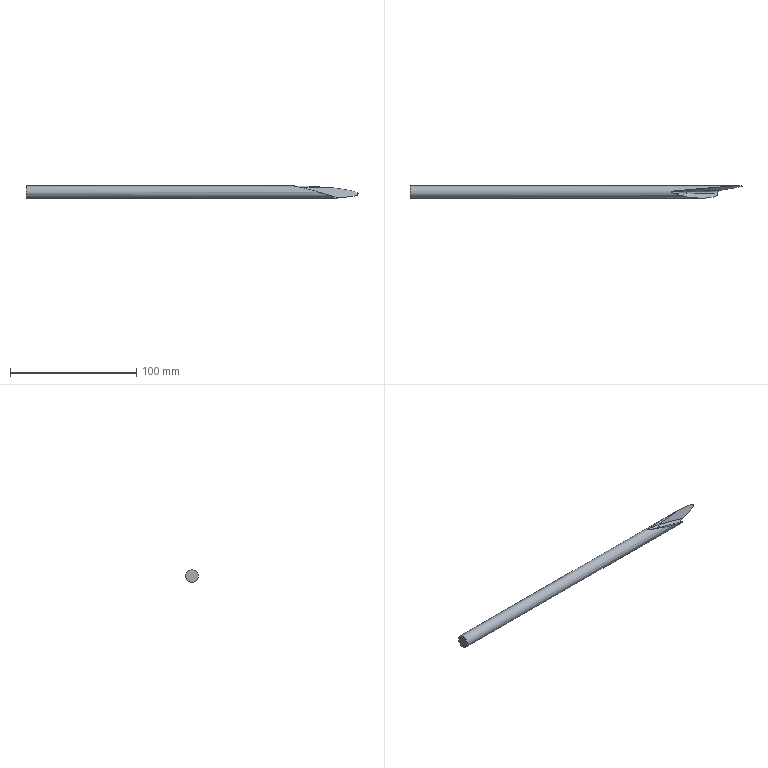Part | STEP file | solid 213 | 1 solid | 7 faces | box 263.363 x 10.007 x 10 mm | volume 18382 mm3 | spline 5 | cylinder 1 | plane 1 | commonest cylinder face diameters 10 x1